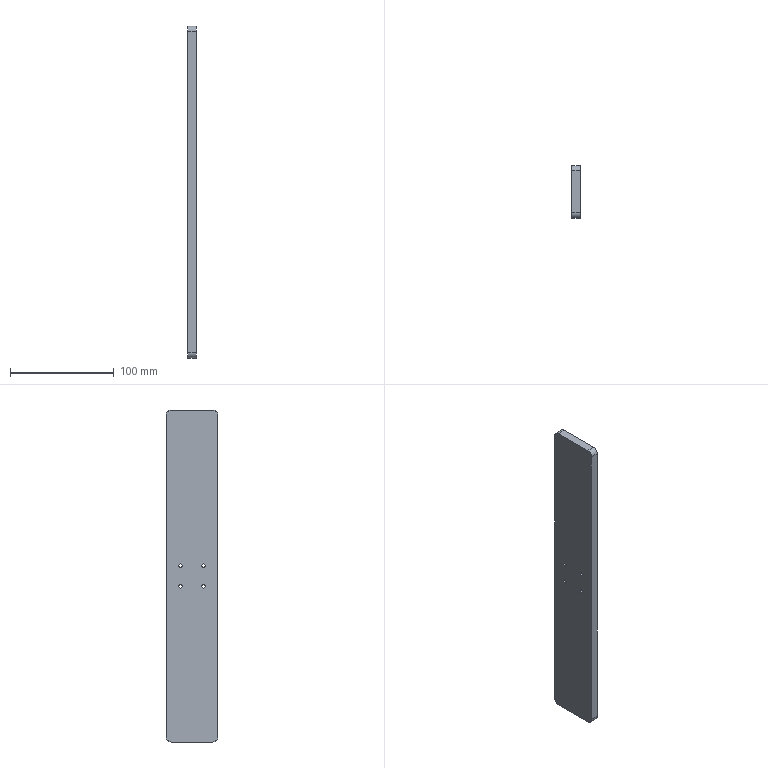Part | SolidWorks | features Extrusion 1, Fillet 1, HoleWzd 1 | 1 solid | 18 faces | box 8 x 50 x 320 mm | volume 127555 mm3 | cylinder 12 | plane 6 | commonest cylinder face diameters 3.3 x8 10 x4
STEP:
#1=CARTESIAN_POINT('',(8.,-11.,-11.65));
#2=VERTEX_POINT('',#1);
#3=CARTESIAN_POINT('',(8.,-11.,-8.35));
#4=VERTEX_POINT('',#3);
#5=CARTESIAN_POINT('',(8.,-11.,-10.));
#6=DIRECTION('',(-1.,0.,0.));
#7=DIRECTION('',(0.,0.,1.));
#8=AXIS2_PLACEMENT_3D('',#5,#6,#7);
#9=CIRCLE('',#8,1.65);
#10=EDGE_CURVE('',#2,#4,#9,.T.);
#11=ORIENTED_EDGE('',*,*,#10,.F.);
#12=CARTESIAN_POINT('',(0.,-11.,-11.65));
#13=VERTEX_POINT('',#12);
#14=CARTESIAN_POINT('',(0.,-11.,-11.65));
#15=DIRECTION('',(-1.,0.,0.));
#16=VECTOR('',#15,1000.);
#17=LINE('',#14,#16);
#18=EDGE_CURVE('',#2,#13,#17,.T.);
#19=ORIENTED_EDGE('',*,*,#18,.T.);
#20=CARTESIAN_POINT('',(0.,-11.,-8.35));
#21=VERTEX_POINT('',#20);
#22=CARTESIAN_POINT('',(0.,-11.,-10.));
#23=DIRECTION('',(-1.,0.,0.));
#24=DIRECTION('',(0.,0.,1.));
#25=AXIS2_PLACEMENT_3D('',#22,#23,#24);
#26=CIRCLE('',#25,1.65);
#27=EDGE_CURVE('',#13,#21,#26,.T.);
#28=ORIENTED_EDGE('',*,*,#27,.T.);
#29=CARTESIAN_POINT('',(0.,-11.,-8.35));
#30=DIRECTION('',(-1.,0.,0.));
#31=VECTOR('',#30,1000.);
#32=LINE('',#29,#31);
#33=EDGE_CURVE('',#4,#21,#32,.T.);
#34=ORIENTED_EDGE('',*,*,#33,.F.);
#35=EDGE_LOOP('',(#11,#19,#28,#34));
#36=FACE_OUTER_BOUND('',#35,.T.);
#37=CARTESIAN_POINT('',(0.,-11.,-10.));
#38=DIRECTION('',(-1.,0.,0.));
#39=DIRECTION('',(0.,0.,1.));
#40=AXIS2_PLACEMENT_3D('',#37,#38,#39);
#41=CYLINDRICAL_SURFACE('',#40,1.65);
#42=ADVANCED_FACE('',(#36),#41,.F.);
#43=CARTESIAN_POINT('',(8.,11.,-11.65));
#44=VERTEX_POINT('',#43);
#45=CARTESIAN_POINT('',(8.,11.,-8.35));
#46=VERTEX_POINT('',#45);
#47=CARTESIAN_POINT('',(8.,11.,-10.));
#48=DIRECTION('',(-1.,0.,0.));
#49=DIRECTION('',(0.,0.,1.));
#50=AXIS2_PLACEMENT_3D('',#47,#48,#49);
#51=CIRCLE('',#50,1.65);
#52=EDGE_CURVE('',#44,#46,#51,.T.);
#53=ORIENTED_EDGE('',*,*,#52,.F.);
#54=CARTESIAN_POINT('',(0.,11.,-11.65));
#55=VERTEX_POINT('',#54);
#56=CARTESIAN_POINT('',(0.,11.,-11.65));
#57=DIRECTION('',(-1.,0.,0.));
#58=VECTOR('',#57,1000.);
#59=LINE('',#56,#58);
#60=EDGE_CURVE('',#44,#55,#59,.T.);
#61=ORIENTED_EDGE('',*,*,#60,.T.);
#62=CARTESIAN_POINT('',(0.,11.,-8.35));
#63=VERTEX_POINT('',#62);
#64=CARTESIAN_POINT('',(0.,11.,-10.));
#65=DIRECTION('',(-1.,0.,0.));
#66=DIRECTION('',(0.,0.,1.));
#67=AXIS2_PLACEMENT_3D('',#64,#65,#66);
#68=CIRCLE('',#67,1.65);
#69=EDGE_CURVE('',#55,#63,#68,.T.);
#70=ORIENTED_EDGE('',*,*,#69,.T.);
#71=CARTESIAN_POINT('',(0.,11.,-8.35));
#72=DIRECTION('',(-1.,0.,0.));
#73=VECTOR('',#72,1000.);
#74=LINE('',#71,#73);
#75=EDGE_CURVE('',#46,#63,#74,.T.);
#76=ORIENTED_EDGE('',*,*,#75,.F.);
#77=EDGE_LOOP('',(#53,#61,#70,#76));
#78=FACE_OUTER_BOUND('',#77,.T.);
#79=CARTESIAN_POINT('',(0.,11.,-10.));
#80=DIRECTION('',(-1.,0.,0.));
#81=DIRECTION('',(0.,0.,1.));
#82=AXIS2_PLACEMENT_3D('',#79,#80,#81);
#83=CYLINDRICAL_SURFACE('',#82,1.65);
#84=ADVANCED_FACE('',(#78),#83,.F.);
#85=CARTESIAN_POINT('',(8.,-11.,8.35));
#86=VERTEX_POINT('',#85);
#87=CARTESIAN_POINT('',(8.,-11.,11.65));
#88=VERTEX_POINT('',#87);
#89=CARTESIAN_POINT('',(8.,-11.,10.));
#90=DIRECTION('',(-1.,0.,0.));
#91=DIRECTION('',(0.,0.,1.));
#92=AXIS2_PLACEMENT_3D('',#89,#90,#91);
#93=CIRCLE('',#92,1.65);
#94=EDGE_CURVE('',#86,#88,#93,.T.);
#95=ORIENTED_EDGE('',*,*,#94,.F.);
#96=CARTESIAN_POINT('',(0.,-11.,8.35));
#97=VERTEX_POINT('',#96);
#98=CARTESIAN_POINT('',(0.,-11.,8.35));
#99=DIRECTION('',(-1.,0.,0.));
#100=VECTOR('',#99,1000.);
#101=LINE('',#98,#100);
#102=EDGE_CURVE('',#86,#97,#101,.T.);
#103=ORIENTED_EDGE('',*,*,#102,.T.);
#104=CARTESIAN_POINT('',(0.,-11.,11.65));
#105=VERTEX_POINT('',#104);
#106=CARTESIAN_POINT('',(0.,-11.,10.));
#107=DIRECTION('',(-1.,0.,0.));
#108=DIRECTION('',(0.,0.,1.));
#109=AXIS2_PLACEMENT_3D('',#106,#107,#108);
#110=CIRCLE('',#109,1.65);
#111=EDGE_CURVE('',#97,#105,#110,.T.);
#112=ORIENTED_EDGE('',*,*,#111,.T.);
#113=CARTESIAN_POINT('',(0.,-11.,11.65));
#114=DIRECTION('',(-1.,0.,0.));
#115=VECTOR('',#114,1000.);
#116=LINE('',#113,#115);
#117=EDGE_CURVE('',#88,#105,#116,.T.);
#118=ORIENTED_EDGE('',*,*,#117,.F.);
#119=EDGE_LOOP('',(#95,#103,#112,#118));
#120=FACE_OUTER_BOUND('',#119,.T.);
#121=CARTESIAN_POINT('',(0.,-11.,10.));
#122=DIRECTION('',(-1.,0.,0.));
#123=DIRECTION('',(0.,0.,1.));
#124=AXIS2_PLACEMENT_3D('',#121,#122,#123);
#125=CYLINDRICAL_SURFACE('',#124,1.65);
#126=ADVANCED_FACE('',(#120),#125,.F.);
#127=CARTESIAN_POINT('',(8.,11.,8.35));
#128=VERTEX_POINT('',#127);
#129=CARTESIAN_POINT('',(8.,11.,11.65));
#130=VERTEX_POINT('',#129);
#131=CARTESIAN_POINT('',(8.,11.,10.));
#132=DIRECTION('',(-1.,0.,0.));
#133=DIRECTION('',(0.,0.,1.));
#134=AXIS2_PLACEMENT_3D('',#131,#132,#133);
#135=CIRCLE('',#134,1.65);
#136=EDGE_CURVE('',#128,#130,#135,.T.);
#137=ORIENTED_EDGE('',*,*,#136,.F.);
#138=CARTESIAN_POINT('',(0.,11.,8.35));
#139=VERTEX_POINT('',#138);
#140=CARTESIAN_POINT('',(0.,11.,8.35));
#141=DIRECTION('',(-1.,0.,0.));
#142=VECTOR('',#141,1000.);
#143=LINE('',#140,#142);
#144=EDGE_CURVE('',#128,#139,#143,.T.);
#145=ORIENTED_EDGE('',*,*,#144,.T.);
#146=CARTESIAN_POINT('',(0.,11.,11.65));
#147=VERTEX_POINT('',#146);
#148=CARTESIAN_POINT('',(0.,11.,10.));
#149=DIRECTION('',(-1.,0.,0.));
#150=DIRECTION('',(0.,0.,1.));
#151=AXIS2_PLACEMENT_3D('',#148,#149,#150);
#152=CIRCLE('',#151,1.65);
#153=EDGE_CURVE('',#139,#147,#152,.T.);
#154=ORIENTED_EDGE('',*,*,#153,.T.);
#155=CARTESIAN_POINT('',(0.,11.,11.65));
#156=DIRECTION('',(-1.,0.,0.));
#157=VECTOR('',#156,1000.);
#158=LINE('',#155,#157);
#159=EDGE_CURVE('',#130,#147,#158,.T.);
#160=ORIENTED_EDGE('',*,*,#159,.F.);
#161=EDGE_LOOP('',(#137,#145,#154,#160));
#162=FACE_OUTER_BOUND('',#161,.T.);
#163=CARTESIAN_POINT('',(0.,11.,10.));
#164=DIRECTION('',(-1.,0.,0.));
#165=DIRECTION('',(0.,0.,1.));
#166=AXIS2_PLACEMENT_3D('',#163,#164,#165);
#167=CYLINDRICAL_SURFACE('',#166,1.65);
#168=ADVANCED_FACE('',(#162),#167,.F.);
#169=CARTESIAN_POINT('',(8.,-20.,-160.));
#170=VERTEX_POINT('',#169);
#171=CARTESIAN_POINT('',(8.,20.,-160.));
#172=VERTEX_POINT('',#171);
#173=CARTESIAN_POINT('',(8.,25.,-160.));
#174=DIRECTION('',(0.,1.,0.));
#175=VECTOR('',#174,1000.);
#176=LINE('',#173,#175);
#177=EDGE_CURVE('',#170,#172,#176,.T.);
#178=ORIENTED_EDGE('',*,*,#177,.F.);
#179=CARTESIAN_POINT('',(0.,-20.,-160.));
#180=VERTEX_POINT('',#179);
#181=CARTESIAN_POINT('',(8.,-20.,-160.));
#182=DIRECTION('',(-1.,0.,0.));
#183=VECTOR('',#182,1000.);
#184=LINE('',#181,#183);
#185=EDGE_CURVE('',#170,#180,#184,.T.);
#186=ORIENTED_EDGE('',*,*,#185,.T.);
#187=CARTESIAN_POINT('',(0.,20.,-160.));
#188=VERTEX_POINT('',#187);
#189=CARTESIAN_POINT('',(0.,25.,-160.));
#190=DIRECTION('',(0.,1.,0.));
#191=VECTOR('',#190,1000.);
#192=LINE('',#189,#191);
#193=EDGE_CURVE('',#180,#188,#192,.T.);
#194=ORIENTED_EDGE('',*,*,#193,.T.);
#195=CARTESIAN_POINT('',(8.,20.,-160.));
#196=DIRECTION('',(1.,0.,0.));
#197=VECTOR('',#196,1000.);
#198=LINE('',#195,#197);
#199=EDGE_CURVE('',#188,#172,#198,.T.);
#200=ORIENTED_EDGE('',*,*,#199,.T.);
#201=EDGE_LOOP('',(#178,#186,#194,#200));
#202=FACE_OUTER_BOUND('',#201,.T.);
#203=CARTESIAN_POINT('',(8.,25.,-160.));
#204=DIRECTION('',(0.,0.,1.));
#205=DIRECTION('',(1.,0.,0.));
#206=AXIS2_PLACEMENT_3D('',#203,#204,#205);
#207=PLANE('',#206);
#208=ADVANCED_FACE('',(#202),#207,.F.);
#209=CARTESIAN_POINT('',(0.,25.,-155.));
#210=VERTEX_POINT('',#209);
#211=CARTESIAN_POINT('',(0.,25.,155.));
#212=VERTEX_POINT('',#211);
#213=CARTESIAN_POINT('',(0.,25.,160.));
#214=DIRECTION('',(0.,0.,1.));
#215=VECTOR('',#214,1000.);
#216=LINE('',#213,#215);
#217=EDGE_CURVE('',#210,#212,#216,.T.);
#218=ORIENTED_EDGE('',*,*,#217,.T.);
#219=CARTESIAN_POINT('',(8.,25.,155.));
#220=VERTEX_POINT('',#219);
#221=CARTESIAN_POINT('',(8.,25.,155.));
#222=DIRECTION('',(1.,0.,0.));
#223=VECTOR('',#222,1000.);
#224=LINE('',#221,#223);
#225=EDGE_CURVE('',#212,#220,#224,.T.);
#226=ORIENTED_EDGE('',*,*,#225,.T.);
#227=CARTESIAN_POINT('',(8.,25.,-155.));
#228=VERTEX_POINT('',#227);
#229=CARTESIAN_POINT('',(8.,25.,160.));
#230=DIRECTION('',(0.,0.,1.));
#231=VECTOR('',#230,1000.);
#232=LINE('',#229,#231);
#233=EDGE_CURVE('',#228,#220,#232,.T.);
#234=ORIENTED_EDGE('',*,*,#233,.F.);
#235=CARTESIAN_POINT('',(8.,25.,-155.));
#236=DIRECTION('',(-1.,0.,0.));
#237=VECTOR('',#236,1000.);
#238=LINE('',#235,#237);
#239=EDGE_CURVE('',#228,#210,#238,.T.);
#240=ORIENTED_EDGE('',*,*,#239,.T.);
#241=EDGE_LOOP('',(#218,#226,#234,#240));
#242=FACE_OUTER_BOUND('',#241,.T.);
#243=CARTESIAN_POINT('',(8.,25.,160.));
#244=DIRECTION('',(0.,-1.,0.));
#245=DIRECTION('',(0.,0.,-1.));
#246=AXIS2_PLACEMENT_3D('',#243,#244,#245);
#247=PLANE('',#246);
#248=ADVANCED_FACE('',(#242),#247,.F.);
#249=CARTESIAN_POINT('',(8.,20.,160.));
#250=VERTEX_POINT('',#249);
#251=CARTESIAN_POINT('',(8.,-20.,160.));
#252=VERTEX_POINT('',#251);
#253=CARTESIAN_POINT('',(8.,25.,160.));
#254=DIRECTION('',(0.,-1.,0.));
#255=VECTOR('',#254,1000.);
#256=LINE('',#253,#255);
#257=EDGE_CURVE('',#250,#252,#256,.T.);
#258=ORIENTED_EDGE('',*,*,#257,.F.);
#259=CARTESIAN_POINT('',(0.,20.,160.));
#260=VERTEX_POINT('',#259);
#261=CARTESIAN_POINT('',(8.,20.,160.));
#262=DIRECTION('',(-1.,0.,0.));
#263=VECTOR('',#262,1000.);
#264=LINE('',#261,#263);
#265=EDGE_CURVE('',#250,#260,#264,.T.);
#266=ORIENTED_EDGE('',*,*,#265,.T.);
#267=CARTESIAN_POINT('',(0.,-20.,160.));
#268=VERTEX_POINT('',#267);
#269=CARTESIAN_POINT('',(0.,25.,160.));
#270=DIRECTION('',(0.,-1.,0.));
#271=VECTOR('',#270,1000.);
#272=LINE('',#269,#271);
#273=EDGE_CURVE('',#260,#268,#272,.T.);
#274=ORIENTED_EDGE('',*,*,#273,.T.);
#275=CARTESIAN_POINT('',(8.,-20.,160.));
#276=DIRECTION('',(1.,0.,0.));
#277=VECTOR('',#276,1000.);
#278=LINE('',#275,#277);
#279=EDGE_CURVE('',#268,#252,#278,.T.);
#280=ORIENTED_EDGE('',*,*,#279,.T.);
#281=EDGE_LOOP('',(#258,#266,#274,#280));
#282=FACE_OUTER_BOUND('',#281,.T.);
#283=CARTESIAN_POINT('',(8.,25.,160.));
#284=DIRECTION('',(0.,0.,-1.));
#285=DIRECTION('',(-1.,0.,0.));
#286=AXIS2_PLACEMENT_3D('',#283,#284,#285);
#287=PLANE('',#286);
#288=ADVANCED_FACE('',(#282),#287,.F.);
#289=CARTESIAN_POINT('',(8.,-25.,155.));
#290=VERTEX_POINT('',#289);
#291=CARTESIAN_POINT('',(8.,-25.,-155.));
#292=VERTEX_POINT('',#291);
#293=CARTESIAN_POINT('',(8.,-25.,160.));
#294=DIRECTION('',(0.,0.,-1.));
#295=VECTOR('',#294,1000.);
#296=LINE('',#293,#295);
#297=EDGE_CURVE('',#290,#292,#296,.T.);
#298=ORIENTED_EDGE('',*,*,#297,.F.);
#299=CARTESIAN_POINT('',(0.,-25.,155.));
#300=VERTEX_POINT('',#299);
#301=CARTESIAN_POINT('',(8.,-25.,155.));
#302=DIRECTION('',(-1.,0.,0.));
#303=VECTOR('',#302,1000.);
#304=LINE('',#301,#303);
#305=EDGE_CURVE('',#290,#300,#304,.T.);
#306=ORIENTED_EDGE('',*,*,#305,.T.);
#307=CARTESIAN_POINT('',(0.,-25.,-155.));
#308=VERTEX_POINT('',#307);
#309=CARTESIAN_POINT('',(0.,-25.,160.));
#310=DIRECTION('',(0.,0.,-1.));
#311=VECTOR('',#310,1000.);
#312=LINE('',#309,#311);
#313=EDGE_CURVE('',#300,#308,#312,.T.);
#314=ORIENTED_EDGE('',*,*,#313,.T.);
#315=CARTESIAN_POINT('',(8.,-25.,-155.));
#316=DIRECTION('',(1.,0.,0.));
#317=VECTOR('',#316,1000.);
#318=LINE('',#315,#317);
#319=EDGE_CURVE('',#308,#292,#318,.T.);
#320=ORIENTED_EDGE('',*,*,#319,.T.);
#321=EDGE_LOOP('',(#298,#306,#314,#320));
#322=FACE_OUTER_BOUND('',#321,.T.);
#323=CARTESIAN_POINT('',(8.,-25.,160.));
#324=DIRECTION('',(0.,1.,0.));
#325=DIRECTION('',(0.,0.,1.));
#326=AXIS2_PLACEMENT_3D('',#323,#324,#325);
#327=PLANE('',#326);
#328=ADVANCED_FACE('',(#322),#327,.F.);
#329=CARTESIAN_POINT('',(8.,-11.,-10.));
#330=DIRECTION('',(-1.,0.,0.));
#331=DIRECTION('',(0.,0.,1.));
#332=AXIS2_PLACEMENT_3D('',#329,#330,#331);
#333=CIRCLE('',#332,1.65);
#334=EDGE_CURVE('',#4,#2,#333,.T.);
#335=ORIENTED_EDGE('',*,*,#334,.T.);
#336=ORIENTED_EDGE('',*,*,#10,.T.);
#337=EDGE_LOOP('',(#335,#336));
#338=FACE_BOUND('',#337,.T.);
#339=CARTESIAN_POINT('',(8.,11.,-10.));
#340=DIRECTION('',(-1.,0.,0.));
#341=DIRECTION('',(0.,0.,1.));
#342=AXIS2_PLACEMENT_3D('',#339,#340,#341);
#343=CIRCLE('',#342,1.65);
#344=EDGE_CURVE('',#46,#44,#343,.T.);
#345=ORIENTED_EDGE('',*,*,#344,.T.);
#346=ORIENTED_EDGE('',*,*,#52,.T.);
#347=EDGE_LOOP('',(#345,#346));
#348=FACE_BOUND('',#347,.T.);
#349=CARTESIAN_POINT('',(8.,-11.,10.));
#350=DIRECTION('',(-1.,0.,0.));
#351=DIRECTION('',(0.,0.,1.));
#352=AXIS2_PLACEMENT_3D('',#349,#350,#351);
#353=CIRCLE('',#352,1.65);
#354=EDGE_CURVE('',#88,#86,#353,.T.);
#355=ORIENTED_EDGE('',*,*,#354,.T.);
#356=ORIENTED_EDGE('',*,*,#94,.T.);
#357=EDGE_LOOP('',(#355,#356));
#358=FACE_BOUND('',#357,.T.);
#359=CARTESIAN_POINT('',(8.,11.,10.));
#360=DIRECTION('',(-1.,0.,0.));
#361=DIRECTION('',(0.,0.,1.));
#362=AXIS2_PLACEMENT_3D('',#359,#360,#361);
#363=CIRCLE('',#362,1.65);
#364=EDGE_CURVE('',#130,#128,#363,.T.);
#365=ORIENTED_EDGE('',*,*,#364,.T.);
#366=ORIENTED_EDGE('',*,*,#136,.T.);
#367=EDGE_LOOP('',(#365,#366));
#368=FACE_BOUND('',#367,.T.);
#369=ORIENTED_EDGE('',*,*,#233,.T.);
#370=CARTESIAN_POINT('',(8.,20.,155.));
#371=DIRECTION('',(1.,0.,0.));
#372=DIRECTION('',(0.,0.,-1.));
#373=AXIS2_PLACEMENT_3D('',#370,#371,#372);
#374=CIRCLE('',#373,5.);
#375=EDGE_CURVE('',#220,#250,#374,.T.);
#376=ORIENTED_EDGE('',*,*,#375,.T.);
#377=ORIENTED_EDGE('',*,*,#257,.T.);
#378=CARTESIAN_POINT('',(8.,-20.,155.));
#379=DIRECTION('',(1.,0.,0.));
#380=DIRECTION('',(0.,0.,-1.));
#381=AXIS2_PLACEMENT_3D('',#378,#379,#380);
#382=CIRCLE('',#381,5.);
#383=EDGE_CURVE('',#252,#290,#382,.T.);
#384=ORIENTED_EDGE('',*,*,#383,.T.);
#385=ORIENTED_EDGE('',*,*,#297,.T.);
#386=CARTESIAN_POINT('',(8.,-20.,-155.));
#387=DIRECTION('',(1.,0.,0.));
#388=DIRECTION('',(0.,0.,-1.));
#389=AXIS2_PLACEMENT_3D('',#386,#387,#388);
#390=CIRCLE('',#389,5.);
#391=EDGE_CURVE('',#292,#170,#390,.T.);
#392=ORIENTED_EDGE('',*,*,#391,.T.);
#393=ORIENTED_EDGE('',*,*,#177,.T.);
#394=CARTESIAN_POINT('',(8.,20.,-155.));
#395=DIRECTION('',(1.,0.,0.));
#396=DIRECTION('',(0.,0.,-1.));
#397=AXIS2_PLACEMENT_3D('',#394,#395,#396);
#398=CIRCLE('',#397,5.);
#399=EDGE_CURVE('',#172,#228,#398,.T.);
#400=ORIENTED_EDGE('',*,*,#399,.T.);
#401=EDGE_LOOP('',(#369,#376,#377,#384,#385,#392,#393,#400));
#402=FACE_OUTER_BOUND('',#401,.T.);
#403=CARTESIAN_POINT('',(8.,0.,0.));
#404=DIRECTION('',(1.,0.,0.));
#405=DIRECTION('',(0.,0.,-1.));
#406=AXIS2_PLACEMENT_3D('',#403,#404,#405);
#407=PLANE('',#406);
#408=ADVANCED_FACE('',(#338,#348,#358,#368,#402),#407,.T.);
#409=CARTESIAN_POINT('',(0.,-11.,-10.));
#410=DIRECTION('',(-1.,0.,0.));
#411=DIRECTION('',(0.,0.,1.));
#412=AXIS2_PLACEMENT_3D('',#409,#410,#411);
#413=CIRCLE('',#412,1.65);
#414=EDGE_CURVE('',#21,#13,#413,.T.);
#415=ORIENTED_EDGE('',*,*,#414,.F.);
#416=ORIENTED_EDGE('',*,*,#27,.F.);
#417=EDGE_LOOP('',(#415,#416));
#418=FACE_BOUND('',#417,.T.);
#419=CARTESIAN_POINT('',(0.,11.,-10.));
#420=DIRECTION('',(-1.,0.,0.));
#421=DIRECTION('',(0.,0.,1.));
#422=AXIS2_PLACEMENT_3D('',#419,#420,#421);
#423=CIRCLE('',#422,1.65);
#424=EDGE_CURVE('',#63,#55,#423,.T.);
#425=ORIENTED_EDGE('',*,*,#424,.F.);
#426=ORIENTED_EDGE('',*,*,#69,.F.);
#427=EDGE_LOOP('',(#425,#426));
#428=FACE_BOUND('',#427,.T.);
#429=CARTESIAN_POINT('',(0.,-11.,10.));
#430=DIRECTION('',(-1.,0.,0.));
#431=DIRECTION('',(0.,0.,1.));
#432=AXIS2_PLACEMENT_3D('',#429,#430,#431);
#433=CIRCLE('',#432,1.65);
#434=EDGE_CURVE('',#105,#97,#433,.T.);
#435=ORIENTED_EDGE('',*,*,#434,.F.);
#436=ORIENTED_EDGE('',*,*,#111,.F.);
#437=EDGE_LOOP('',(#435,#436));
#438=FACE_BOUND('',#437,.T.);
#439=CARTESIAN_POINT('',(0.,11.,10.));
#440=DIRECTION('',(-1.,0.,0.));
#441=DIRECTION('',(0.,0.,1.));
#442=AXIS2_PLACEMENT_3D('',#439,#440,#441);
#443=CIRCLE('',#442,1.65);
#444=EDGE_CURVE('',#147,#139,#443,.T.);
#445=ORIENTED_EDGE('',*,*,#444,.F.);
#446=ORIENTED_EDGE('',*,*,#153,.F.);
#447=EDGE_LOOP('',(#445,#446));
#448=FACE_BOUND('',#447,.T.);
#449=ORIENTED_EDGE('',*,*,#273,.F.);
#450=CARTESIAN_POINT('',(0.,20.,155.));
#451=DIRECTION('',(-1.,0.,0.));
#452=DIRECTION('',(0.,0.,-1.));
#453=AXIS2_PLACEMENT_3D('',#450,#451,#452);
#454=CIRCLE('',#453,5.);
#455=EDGE_CURVE('',#260,#212,#454,.T.);
#456=ORIENTED_EDGE('',*,*,#455,.T.);
#457=ORIENTED_EDGE('',*,*,#217,.F.);
#458=CARTESIAN_POINT('',(0.,20.,-155.));
#459=DIRECTION('',(-1.,0.,0.));
#460=DIRECTION('',(0.,0.,-1.));
#461=AXIS2_PLACEMENT_3D('',#458,#459,#460);
#462=CIRCLE('',#461,5.);
#463=EDGE_CURVE('',#210,#188,#462,.T.);
#464=ORIENTED_EDGE('',*,*,#463,.T.);
#465=ORIENTED_EDGE('',*,*,#193,.F.);
#466=CARTESIAN_POINT('',(0.,-20.,-155.));
#467=DIRECTION('',(-1.,0.,0.));
#468=DIRECTION('',(0.,0.,-1.));
#469=AXIS2_PLACEMENT_3D('',#466,#467,#468);
#470=CIRCLE('',#469,5.);
#471=EDGE_CURVE('',#180,#308,#470,.T.);
#472=ORIENTED_EDGE('',*,*,#471,.T.);
#473=ORIENTED_EDGE('',*,*,#313,.F.);
#474=CARTESIAN_POINT('',(0.,-20.,155.));
#475=DIRECTION('',(-1.,0.,0.));
#476=DIRECTION('',(0.,0.,-1.));
#477=AXIS2_PLACEMENT_3D('',#474,#475,#476);
#478=CIRCLE('',#477,5.);
#479=EDGE_CURVE('',#300,#268,#478,.T.);
#480=ORIENTED_EDGE('',*,*,#479,.T.);
#481=EDGE_LOOP('',(#449,#456,#457,#464,#465,#472,#473,#480));
#482=FACE_OUTER_BOUND('',#481,.T.);
#483=CARTESIAN_POINT('',(0.,0.,0.));
#484=DIRECTION('',(1.,0.,0.));
#485=DIRECTION('',(0.,0.,-1.));
#486=AXIS2_PLACEMENT_3D('',#483,#484,#485);
#487=PLANE('',#486);
#488=ADVANCED_FACE('',(#418,#428,#438,#448,#482),#487,.F.);
#489=ORIENTED_EDGE('',*,*,#144,.F.);
#490=ORIENTED_EDGE('',*,*,#364,.F.);
#491=ORIENTED_EDGE('',*,*,#159,.T.);
#492=ORIENTED_EDGE('',*,*,#444,.T.);
#493=EDGE_LOOP('',(#489,#490,#491,#492));
#494=FACE_OUTER_BOUND('',#493,.T.);
#495=CARTESIAN_POINT('',(0.,11.,10.));
#496=DIRECTION('',(-1.,0.,0.));
#497=DIRECTION('',(0.,0.,1.));
#498=AXIS2_PLACEMENT_3D('',#495,#496,#497);
#499=CYLINDRICAL_SURFACE('',#498,1.65);
#500=ADVANCED_FACE('',(#494),#499,.F.);
#501=ORIENTED_EDGE('',*,*,#102,.F.);
#502=ORIENTED_EDGE('',*,*,#354,.F.);
#503=ORIENTED_EDGE('',*,*,#117,.T.);
#504=ORIENTED_EDGE('',*,*,#434,.T.);
#505=EDGE_LOOP('',(#501,#502,#503,#504));
#506=FACE_OUTER_BOUND('',#505,.T.);
#507=CARTESIAN_POINT('',(0.,-11.,10.));
#508=DIRECTION('',(-1.,0.,0.));
#509=DIRECTION('',(0.,0.,1.));
#510=AXIS2_PLACEMENT_3D('',#507,#508,#509);
#511=CYLINDRICAL_SURFACE('',#510,1.65);
#512=ADVANCED_FACE('',(#506),#511,.F.);
#513=ORIENTED_EDGE('',*,*,#60,.F.);
#514=ORIENTED_EDGE('',*,*,#344,.F.);
#515=ORIENTED_EDGE('',*,*,#75,.T.);
#516=ORIENTED_EDGE('',*,*,#424,.T.);
#517=EDGE_LOOP('',(#513,#514,#515,#516));
#518=FACE_OUTER_BOUND('',#517,.T.);
#519=CARTESIAN_POINT('',(0.,11.,-10.));
#520=DIRECTION('',(-1.,0.,0.));
#521=DIRECTION('',(0.,0.,1.));
#522=AXIS2_PLACEMENT_3D('',#519,#520,#521);
#523=CYLINDRICAL_SURFACE('',#522,1.65);
#524=ADVANCED_FACE('',(#518),#523,.F.);
#525=ORIENTED_EDGE('',*,*,#18,.F.);
#526=ORIENTED_EDGE('',*,*,#334,.F.);
#527=ORIENTED_EDGE('',*,*,#33,.T.);
#528=ORIENTED_EDGE('',*,*,#414,.T.);
#529=EDGE_LOOP('',(#525,#526,#527,#528));
#530=FACE_OUTER_BOUND('',#529,.T.);
#531=CARTESIAN_POINT('',(0.,-11.,-10.));
#532=DIRECTION('',(-1.,0.,0.));
#533=DIRECTION('',(0.,0.,1.));
#534=AXIS2_PLACEMENT_3D('',#531,#532,#533);
#535=CYLINDRICAL_SURFACE('',#534,1.65);
#536=ADVANCED_FACE('',(#530),#535,.F.);
#537=ORIENTED_EDGE('',*,*,#375,.F.);
#538=ORIENTED_EDGE('',*,*,#225,.F.);
#539=ORIENTED_EDGE('',*,*,#455,.F.);
#540=ORIENTED_EDGE('',*,*,#265,.F.);
#541=EDGE_LOOP('',(#537,#538,#539,#540));
#542=FACE_OUTER_BOUND('',#541,.T.);
#543=CARTESIAN_POINT('',(8.,20.,155.));
#544=DIRECTION('',(-1.,0.,0.));
#545=DIRECTION('',(0.,0.,1.));
#546=AXIS2_PLACEMENT_3D('',#543,#544,#545);
#547=CYLINDRICAL_SURFACE('',#546,5.);
#548=ADVANCED_FACE('',(#542),#547,.T.);
#549=ORIENTED_EDGE('',*,*,#383,.F.);
#550=ORIENTED_EDGE('',*,*,#279,.F.);
#551=ORIENTED_EDGE('',*,*,#479,.F.);
#552=ORIENTED_EDGE('',*,*,#305,.F.);
#553=EDGE_LOOP('',(#549,#550,#551,#552));
#554=FACE_OUTER_BOUND('',#553,.T.);
#555=CARTESIAN_POINT('',(8.,-20.,155.));
#556=DIRECTION('',(-1.,0.,0.));
#557=DIRECTION('',(0.,0.,1.));
#558=AXIS2_PLACEMENT_3D('',#555,#556,#557);
#559=CYLINDRICAL_SURFACE('',#558,5.);
#560=ADVANCED_FACE('',(#554),#559,.T.);
#561=ORIENTED_EDGE('',*,*,#391,.F.);
#562=ORIENTED_EDGE('',*,*,#319,.F.);
#563=ORIENTED_EDGE('',*,*,#471,.F.);
#564=ORIENTED_EDGE('',*,*,#185,.F.);
#565=EDGE_LOOP('',(#561,#562,#563,#564));
#566=FACE_OUTER_BOUND('',#565,.T.);
#567=CARTESIAN_POINT('',(8.,-20.,-155.));
#568=DIRECTION('',(-1.,0.,0.));
#569=DIRECTION('',(0.,0.,1.));
#570=AXIS2_PLACEMENT_3D('',#567,#568,#569);
#571=CYLINDRICAL_SURFACE('',#570,5.);
#572=ADVANCED_FACE('',(#566),#571,.T.);
#573=ORIENTED_EDGE('',*,*,#399,.F.);
#574=ORIENTED_EDGE('',*,*,#199,.F.);
#575=ORIENTED_EDGE('',*,*,#463,.F.);
#576=ORIENTED_EDGE('',*,*,#239,.F.);
#577=EDGE_LOOP('',(#573,#574,#575,#576));
#578=FACE_OUTER_BOUND('',#577,.T.);
#579=CARTESIAN_POINT('',(8.,20.,-155.));
#580=DIRECTION('',(-1.,0.,0.));
#581=DIRECTION('',(0.,0.,1.));
#582=AXIS2_PLACEMENT_3D('',#579,#580,#581);
#583=CYLINDRICAL_SURFACE('',#582,5.);
#584=ADVANCED_FACE('',(#578),#583,.T.);
#585=CLOSED_SHELL('',(#42,#84,#126,#168,#208,#248,#288,#328,#408,#488,#500,#512,#524,#536,#548,#560,#572,#584));
#586=MANIFOLD_SOLID_BREP('',#585);
#587=CARTESIAN_POINT('',(0.,0.,0.));
#588=DIRECTION('',(0.,0.,1.));
#589=DIRECTION('',(1.,0.,0.));
#590=AXIS2_PLACEMENT_3D('',#587,#588,#589);
#591=(LENGTH_UNIT()NAMED_UNIT(*)SI_UNIT(.MILLI.,.METRE.));
#592=UNCERTAINTY_MEASURE_WITH_UNIT(LENGTH_MEASURE(0.00001),#591,'','');
#593=(NAMED_UNIT(*)PLANE_ANGLE_UNIT()SI_UNIT($,.RADIAN.));
#594=(NAMED_UNIT(*)SI_UNIT($,.STERADIAN.)SOLID_ANGLE_UNIT());
#595=(GEOMETRIC_REPRESENTATION_CONTEXT(3)GLOBAL_UNCERTAINTY_ASSIGNED_CONTEXT((#592))GLOBAL_UNIT_ASSIGNED_CONTEXT((#591,#593,#594))REPRESENTATION_CONTEXT('',''));
#596=ADVANCED_BREP_SHAPE_REPRESENTATION('',(#586,#590),#595);